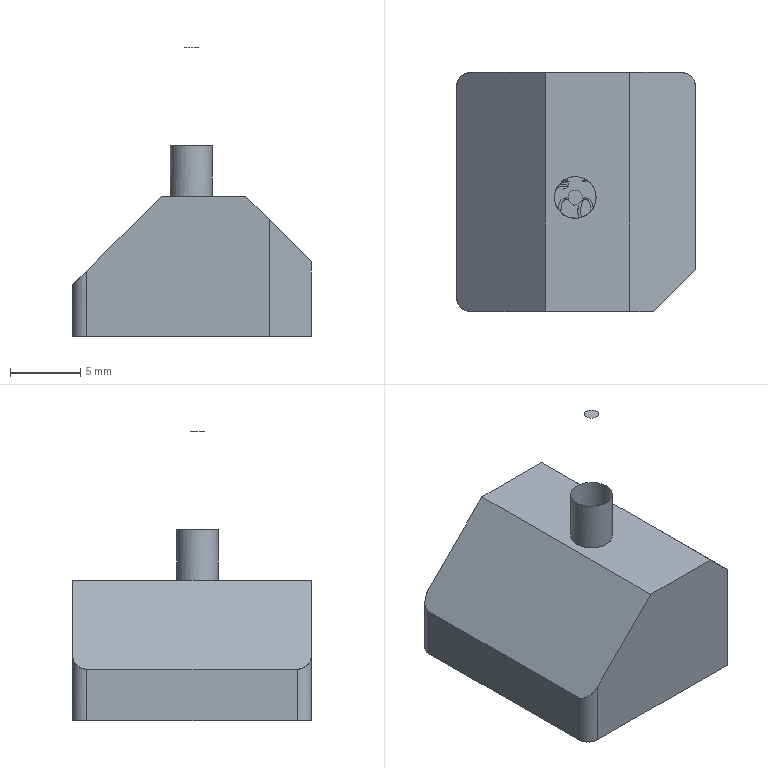NC program | PowerMill | posted with a generic post | part box 17 x 17 x 20.603 mm
Lines 3444 to 3961 of 42778:
N3541 M6
N3542 S8500 M03
N3543 G00 G90 X0.002 Y0.0
N3544 G43 Z11.803 H3
N3545
N3546 G05 P10000 R8
N3547 X6.5189 Y8.6331
N3548 Z0.8529
N3549 G01 Z-0.3471 F360.0
N3550 X3.4666 Y4.3309 F600.0
N3551 X-5.7661 Y-1.8674
N3552 X-5.6728 Y-2.1912
N3553 X-5.4516 Y-2.7818
N3554 X-5.3113 Y-3.0682
N3555 X-5.1953 Y-3.2909
N3556 X-4.9958 Y-3.6229
N3557 X-4.6728 Y-4.0697
N3558 X-4.5415 Y-4.2305
N3559 X-4.2593 Y-4.5375
N3560 G03 X-3.6303 Y-5.092 I4.7377 J4.7404
N3561 G01 X-3.5719 Y-5.1319
N3562 X5.661 Y1.0665
N3563 G00 Z11.803
N3564 G05 P0
N3565 (---------------)
N3566 ( END TOOLPATH : 粗公基准台01-平坦面平行-D10 )
N3567 (---------------)
N3568 ( START TOOLPATH : 粗公基准台01-基准面偏置-D10 )
N3569 (---------------)
N3570 G00 X0.002 Y0.0 Z9.8029
N3571 G05 P10000 R8
N3572 X-2.4609 Y19.1679
N3573 Z-9.6
N3574 G01 Z-10.8 F360.0
N3575 X-2.2639 Y13.8966 F600.0
N3576 X-5.1039 Y4.1284
N3577 G02 X-4.3127 Y4.8796 I6.1923 J-5.7295
N3578 G01 X-4.0577 Y5.0698
N3579 X-3.5215 Y5.4298
N3580 X-3.1259 Y5.6451
N3581 X-2.7927 Y5.8019
N3582 G02 X-2.3057 Y5.99 I1.3954 J-2.888
N3583 G01 X-1.9392 Y6.1117
N3584 G02 X-1.148 Y6.2935 I1.8874 J-6.3997
N3585 G01 X-0.3568 Y6.3775
N3586 X0.4344 Y6.3644
N3587 X0.83 Y6.3263
N3588 X1.2256 Y6.2581
N3589 G02 X2.0168 Y6.06 I-1.3394 J-7.0312
N3590 G01 X2.415 Y5.9128
N3591 X2.808 Y5.7518
N3592 X3.2036 Y5.548
N3593 X3.5992 Y5.3157
N3594 X3.8789 Y5.1285
N3595 X4.3904 Y4.724
N3596 X4.5997 Y4.5366
N3597 X4.7999 Y4.3395
N3598 X5.1816 Y3.9134
N3599 X5.462 Y3.5505
N3600 X5.72 Y3.156
N3601 X5.9727 Y2.7176
N3602 X6.3019 Y1.9725
N3603 X6.4361 Y1.578
N3604 X6.5399 Y1.1835
N3605 X6.6264 Y0.789
N3606 X6.6836 Y0.3945
N3607 X6.7315 Y-0.3945
N3608 X6.6843 Y-1.1835
N3609 X6.6285 Y-1.578
N3610 X6.5422 Y-1.9725
N3611 X6.4395 Y-2.367
N3612 X6.3065 Y-2.7615
N3613 X5.9557 Y-3.5505
N3614 X5.7269 Y-3.945
N3615 X5.4697 Y-4.3395
N3616 X5.1815 Y-4.7132
N3617 X4.8107 Y-5.1285
N3618 X4.6054 Y-5.3313
N3619 X4.3904 Y-5.5238
N3620 X3.8943 Y-5.9175
N3621 X3.5992 Y-6.1163
N3622 G02 X2.808 Y-6.5516 I-4.9668 J8.09
N3623 G01 X2.4155 Y-6.7137
N3624 X2.0168 Y-6.8598
N3625 X1.6212 Y-6.9736
N3626 X1.2256 Y-7.0586
N3627 X0.83 Y-7.1267
N3628 X0.4344 Y-7.1642
N3629 X-0.3568 Y-7.1773
N3630 X-1.148 Y-7.0933
N3631 G02 X-2.1733 Y-6.8331 I0.9602 J5.9347
N3632 G01 X-2.5519 Y-6.7065
N3633 X-3.126 Y-6.4452
N3634 X-3.5215 Y-6.2296
N3635 X-3.9929 Y-5.9175
N3636 X-4.3128 Y-5.6794
N3637 X-4.6133 Y-5.4182
N3638 X-4.9139 Y-5.1285
N3639 G02 X-5.5147 Y-4.4156 I4.536 J4.4326
N3640 G01 X-5.6438 Y-4.2299
N3641 X-5.8951 Y-3.8456
N3642 X-6.0842 Y-3.4937
N3643 X-6.2596 Y-3.1348
N3644 X-6.4097 Y-2.7615
N3645 X-6.5425 Y-2.367
N3646 X-6.6515 Y-1.9725
N3647 X-6.6863 Y-1.8138
N3648 X-6.7899 Y-1.1835
N3649 X-6.8246 Y-0.789
N3650 X-6.8313 Y-0.3945
N3651 X-6.8246 Y0.0
N3652 X-6.7883 Y0.3945
N3653 X-6.6767 Y1.064
N3654 X-6.5387 Y1.578
N3655 G02 X-6.2464 Y2.367 I7.6007 J-2.3668
N3656 G01 X-6.0757 Y2.709
N3657 X-5.8951 Y3.0458
N3658 X-5.7359 Y3.3024
N3659 X-5.5637 Y3.5505
N3660 X-5.3461 Y3.8394
N3661 X-5.1039 Y4.1284
N3662 G00 Z9.8029
N3663 G05 P0
N3664 (---------------)
N3665 ( END TOOLPATH : 粗公基准台01-基准面偏置-D10 )
N3666 (---------------)
N3667 ( START TOOLPATH : 粗公基准台01-基准台侧光-D10 )
N3668 (---------------)
N3669 G00 X0.002 Y0.0 Z9.8029
N3670 G05 P10000 R8
N3671 X13.4802 Y-14.7763
N3672 Z-19.5
N3673 G01 Z-20.7 F360.0
N3674 G03 X9.9447 Y-11.2408 I-1.7677 J1.7678 F600.0
N3675 G01 X9.0603 Y-12.1252
N3676 X9.0598 Y-12.1257
N3677 X9.0593 Y-12.1262
N3678 X8.9973 Y-12.186
N3679 X8.9953 Y-12.1879
N3680 X8.9933 Y-12.1896
N3681 X8.5463 Y-12.5663
N3682 X8.5428 Y-12.5691
N3683 X8.5391 Y-12.5717
N3684 X8.0921 Y-12.8697
N3685 X8.0892 Y-12.8716
N3686 X8.0862 Y-12.8734
N3687 X7.7951 Y-13.0328
N3688 X7.7933 Y-13.0337
N3689 X7.7915 Y-13.0346
N3690 X7.6356 Y-13.11
N3691 X7.6332 Y-13.1111
N3692 X7.6308 Y-13.1122
N3693 X7.1838 Y-13.2933
N3694 X7.1803 Y-13.2947
N3695 X7.1766 Y-13.2958
N3696 X6.7297 Y-13.4292
N3697 X6.7268 Y-13.43
N3698 X6.724 Y-13.4307
N3699 X6.4655 Y-13.4877
N3700 X6.4637 Y-13.4881
N3701 X6.4619 Y-13.4884
N3702 X6.2734 Y-13.521
N3703 X6.2709 Y-13.5214
N3704 X6.2684 Y-13.5217
N3705 X5.8214 Y-13.5699
N3706 X5.818 Y-13.5702
N3707 X5.8146 Y-13.5703
N3708 X5.3676 Y-13.58
N3709 X5.3667
N3710 X5.3658
N3711 X-7.5968 Y-13.5791
N3712 X-7.599 Y-13.579
N3713 X-7.6012 Y-13.5789
N3714 X-8.0482 Y-13.5541
N3715 X-8.0511 Y-13.5539
N3716 X-8.0539 Y-13.5536
N3717 X-8.5009 Y-13.4962
N3718 X-8.5039 Y-13.4958
N3719 X-8.5069 Y-13.4952
N3720 X-8.9539 Y-13.403
N3721 X-8.957 Y-13.4023
N3722 X-8.9601 Y-13.4014
N3723 X-9.4071 Y-13.271
N3724 X-9.4099 Y-13.2702
N3725 X-9.4126 Y-13.2692
N3726 X-9.8596 Y-13.1027
N3727 X-9.8628 Y-13.1014
N3728 X-9.866 Y-13.1
N3729 X-10.3129 Y-12.8881
N3730 X-10.3158 Y-12.8867
N3731 X-10.3186 Y-12.8851
N3732 X-10.7656 Y-12.6274
N3733 X-10.7687 Y-12.6256
N3734 X-10.7717 Y-12.6235
N3735 X-11.2187 Y-12.3088
N3736 X-11.2209 Y-12.3072
N3737 X-11.2231 Y-12.3055
N3738 X-11.4383 Y-12.1307
N3739 X-11.4399 Y-12.1294
N3740 X-11.4414 Y-12.1281
N3741 X-11.6731 Y-11.9195
N3742 X-11.6747 Y-11.9181
N3743 X-11.6762 Y-11.9166
N3744 X-11.9146 Y-11.6782
N3745 X-11.9161 Y-11.6767
N3746 X-11.9175 Y-11.6751
N3747 X-12.1261 Y-11.4435
N3748 X-12.1274 Y-11.4419
N3749 X-12.1287 Y-11.4404
N3750 X-12.3036 Y-11.2251
N3751 X-12.3052 Y-11.2231
N3752 X-12.3066 Y-11.2211
N3753 X-12.5787 Y-10.8401
N3754 X-12.5807 Y-10.8371
N3755 X-12.5826 Y-10.834
N3756 X-12.8831 Y-10.3211
N3757 X-12.8848 Y-10.3181
N3758 X-12.8863 Y-10.3149
N3759 X-13.0983 Y-9.868
N3760 X-13.0997 Y-9.8648
N3761 X-13.1009 Y-9.8616
N3762 X-13.2675 Y-9.4146
N3763 X-13.2685 Y-9.4119
N3764 X-13.2693 Y-9.4091
N3765 X-13.3997 Y-8.9621
N3766 X-13.4005 Y-8.9592
N3767 X-13.4012 Y-8.9562
N3768 X-13.4858 Y-8.555
N3769 X-13.4864 Y-8.552
N3770 X-13.4869 Y-8.549
N3771 X-13.552 Y-8.0562
N3772 X-13.5523 Y-8.0532
N3773 X-13.5525 Y-8.0502
N3774 X-13.5774 Y-7.6032
N3775 X-13.5775 Y-7.601
N3776 Y-7.5988
N3777 Y7.5988
N3778 Y7.601
N3779 X-13.5774 Y7.6032
N3780 X-13.5525 Y8.0502
N3781 X-13.5523 Y8.0531
N3782 X-13.552 Y8.0559
N3783 X-13.4946 Y8.5029
N3784 X-13.4941 Y8.5059
N3785 X-13.4936 Y8.5089
N3786 X-13.4013 Y8.9559
N3787 X-13.4005 Y8.959
N3788 X-13.3997 Y8.9621
N3789 X-13.2693 Y9.4091
N3790 X-13.2685 Y9.4119
N3791 X-13.2675 Y9.4146
N3792 X-13.1009 Y9.8616
N3793 X-13.0997 Y9.8648
N3794 X-13.0983 Y9.868
N3795 X-12.8863 Y10.3149
N3796 X-12.8849 Y10.3178
N3797 X-12.8834 Y10.3206
N3798 X-12.6256 Y10.7676
N3799 X-12.6237 Y10.7707
N3800 X-12.6217 Y10.7737
N3801 X-12.3069 Y11.2207
N3802 X-12.3053 Y11.2229
N3803 X-12.3036 Y11.2251
N3804 X-12.1287 Y11.4404
N3805 X-12.1274 Y11.4419
N3806 X-12.1261 Y11.4435
N3807 X-11.9175 Y11.6751
N3808 X-11.9161 Y11.6767
N3809 X-11.9146 Y11.6782
N3810 X-11.6762 Y11.9166
N3811 X-11.6747 Y11.9181
N3812 X-11.6731 Y11.9195
N3813 X-11.4414 Y12.1281
N3814 X-11.4399 Y12.1294
N3815 X-11.4383 Y12.1307
N3816 X-11.2231 Y12.3055
N3817 X-11.2211 Y12.3071
N3818 X-11.2191 Y12.3085
N3819 X-10.8379 Y12.5807
N3820 X-10.8349 Y12.5827
N3821 X-10.8318 Y12.5846
N3822 X-10.3191 Y12.8849
N3823 X-10.3161 Y12.8865
N3824 X-10.3129 Y12.8881
N3825 X-9.866 Y13.1
N3826 X-9.8628 Y13.1014
N3827 X-9.8596 Y13.1027
N3828 X-9.4126 Y13.2692
N3829 X-9.4099 Y13.2702
N3830 X-9.4071 Y13.271
N3831 X-8.9601 Y13.4014
N3832 X-8.9572 Y13.4022
N3833 X-8.9542 Y13.4029
N3834 X-8.5509 Y13.4879
N3835 X-8.5479 Y13.4884
N3836 X-8.5449 Y13.4889
N3837 X-8.0542 Y13.5535
N3838 X-8.0512 Y13.5539
N3839 X-8.0482 Y13.5541
N3840 X-7.6012 Y13.579
N3841 X-7.599 Y13.5791
N3842 X-7.5968
N3843 X0.002
N3844 X7.6008 Y13.579
N3845 X7.603
N3846 X7.6052 Y13.5789
N3847 X8.0522 Y13.5541
N3848 X8.0551 Y13.5538
N3849 X8.0579 Y13.5535
N3850 X8.5049 Y13.4961
N3851 X8.5079 Y13.4956
N3852 X8.5109 Y13.4951
N3853 X8.9579 Y13.4027
N3854 X8.961 Y13.402
N3855 X8.9641 Y13.4012
N3856 X9.4111 Y13.2707
N3857 X9.4139 Y13.2699
N3858 X9.4166 Y13.2689
N3859 X9.8636 Y13.1024
N3860 X9.8668 Y13.1011
N3861 X9.87 Y13.0997
N3862 X10.317 Y12.8876
N3863 X10.3198 Y12.8862
N3864 X10.3226 Y12.8847
N3865 X10.7696 Y12.6269
N3866 X10.7727 Y12.625
N3867 X10.7757 Y12.623
N3868 X11.2227 Y12.3082
N3869 X11.2249 Y12.3066
N3870 X11.2271 Y12.3049
N3871 X11.4415 Y12.1307
N3872 X11.443 Y12.1294
N3873 X11.4446 Y12.1281
N3874 X11.6771 Y11.9187
N3875 X11.6787 Y11.9173
N3876 X11.6802 Y11.9158
N3877 X11.9178 Y11.6782
N3878 X11.9193 Y11.6767
N3879 X11.9207 Y11.6751
N3880 X12.1301 Y11.4424
N3881 X12.1314 Y11.4409
N3882 X12.1327 Y11.4394
N3883 X12.3068 Y11.2251
N3884 X12.3083 Y11.2231
N3885 X12.3098 Y11.2211
N3886 X12.5827 Y10.8388
N3887 X12.5847 Y10.8358
N3888 X12.5866 Y10.8327
N3889 X12.8862 Y10.3211
N3890 X12.8879 Y10.3181
N3891 X12.8895 Y10.3149
N3892 X13.1014 Y9.868
N3893 X13.1028 Y9.8648
N3894 X13.1041 Y9.8616
N3895 X13.2706 Y9.4146
N3896 X13.2716 Y9.4119
N3897 X13.2725 Y9.4091
N3898 X13.4029 Y8.9621
N3899 X13.4037 Y8.9592
N3900 X13.4044 Y8.9562
N3901 X13.4899 Y8.55
N3902 X13.4904 Y8.547
N3903 X13.4909 Y8.5439
N3904 X13.5551 Y8.0562
N3905 X13.5554 Y8.0532
N3906 X13.5556 Y8.0502
N3907 X13.5805 Y7.6032
N3908 X13.5806 Y7.601
N3909 Y7.5988
N3910 X13.5816 Y-5.3638
N3911 Y-5.3647
N3912 Y-5.3656
N3913 X13.5719 Y-5.8126
N3914 X13.5717 Y-5.816
N3915 X13.5715 Y-5.8194
N3916 X13.5234 Y-6.2664
N3917 X13.5231 Y-6.2689
N3918 X13.5227 Y-6.2714
N3919 X13.4904 Y-6.4581
N3920 X13.4901 Y-6.4599
N3921 X13.4897 Y-6.4616
N3922 X13.4324 Y-6.722
N3923 X13.4317 Y-6.7248
N3924 X13.431 Y-6.7277
N3925 X13.2975 Y-7.1747
N3926 X13.2964 Y-7.1783
N3927 X13.295 Y-7.1818
N3928 X13.1139 Y-7.6288
N3929 X13.1129 Y-7.6312
N3930 X13.1118 Y-7.6336
N3931 X13.0366 Y-7.7891
N3932 X13.0357 Y-7.7909
N3933 X13.0348 Y-7.7926
N3934 X12.8752 Y-8.0842
N3935 X12.8735 Y-8.0871
N3936 X12.8716 Y-8.09
N3937 X12.5842 Y-8.5228
N3938 X12.5817 Y-8.5265
N3939 X12.5789 Y-8.53
N3940 X12.1917 Y-8.9912
N3941 X12.1899 Y-8.9932
N3942 X12.188 Y-8.9953
N3943 X12.1282 Y-9.0573
N3944 X12.1277 Y-9.0578
N3945 X12.1272 Y-9.0583
N3946 X9.9447 Y-11.2408
N3947 G03 X13.4802 Y-14.7763 I1.7678 J-1.7677
N3948 G01 X13.4288 Y-14.7146
N3949 G03 X9.8932 Y-11.1791 I-1.7678 J1.7677
N3950 G01 X9.0037 Y-12.0686
N3951 X8.9417 Y-12.1285
N3952 X8.4947 Y-12.5052
N3953 X8.0477 Y-12.8032
N3954 X7.7566 Y-12.9626
N3955 X7.6008 Y-13.038
N3956 X7.1538 Y-13.2192
N3957 X6.7068 Y-13.3526
N3958 X6.4482 Y-13.4096
N3959 X6.2598 Y-13.4422
N3960 X5.8128 Y-13.4903
N3961 X5.3658 Y-13.5
N3962 X-7.5968 Y-13.4991
N3963 X-8.0437 Y-13.4742
N3964 X-8.4907 Y-13.4169
N3965 X-8.9377 Y-13.3246
N3966 X-9.3847 Y-13.1942
N3967 X-9.8317 Y-13.0277
N3968 X-10.2787 Y-12.8158
N3969 X-10.7257 Y-12.5581
N3970 X-11.1726 Y-12.2434
N3971 X-11.3879 Y-12.0686
N3972 X-11.6196 Y-11.8601
N3973 X-11.8581 Y-11.6216
N3974 X-12.0666 Y-11.3899
N3975 X-12.2415 Y-11.1746
N3976 X-12.5136 Y-10.7936
N3977 X-12.8141 Y-10.2807
N3978 X-13.026 Y-9.8337
N3979 X-13.1925 Y-9.3867
N3980 X-13.3229 Y-8.9397
N3981 X-13.4076 Y-8.5385
N3982 X-13.4726 Y-8.0457
N3983 X-13.4975 Y-7.5988
N3984 Y7.5988
N3985 X-13.4726 Y8.0457
N3986 X-13.4152 Y8.4927
N3987 X-13.3229 Y8.9397
N3988 X-13.1925 Y9.3867
N3989 X-13.026 Y9.8337
N3990 X-12.8141 Y10.2807
N3991 X-12.5563 Y10.7277
N3992 X-12.2415 Y11.1746
N3993 X-12.0666 Y11.3899
N3994 X-11.8581 Y11.6216
N3995 X-11.6196 Y11.8601
N3996 X-11.3879 Y12.0686
N3997 X-11.1726 Y12.2434
N3998 X-10.7914 Y12.5156
N3999 X-10.2787 Y12.8158
N4000 X-9.8317 Y13.0277
N4001 X-9.3847 Y13.1942
N4002 X-8.9377 Y13.3246
N4003 X-8.5344 Y13.4096
N4004 X-8.0437 Y13.4742
N4005 X-7.5968 Y13.4991
N4006 X0.002
N4007 X7.6008 Y13.499
N4008 X8.0477 Y13.4742
N4009 X8.4947 Y13.4167
N4010 X8.9417 Y13.3244
N4011 X9.3887 Y13.1939
N4012 X9.8357 Y13.0274
N4013 X10.2827 Y12.8154
N4014 X10.7297 Y12.5576
N4015 X11.1766 Y12.2428
N4016 X11.391 Y12.0686
N4017 X11.6236 Y11.8593
N4018 X11.8612 Y11.6216
N4019 X12.0706 Y11.3889
N4020 X12.2447 Y11.1746
N4021 X12.5176 Y10.7923
N4022 X12.8172 Y10.2807
N4023 X13.0291 Y9.8337
N4024 X13.1957 Y9.3867
N4025 X13.3261 Y8.9397
N4026 X13.4116 Y8.5335
N4027 X13.4758 Y8.0457
N4028 X13.5006 Y7.5988
N4029 X13.5016 Y-5.3638
N4030 X13.4919 Y-5.8108
N4031 X13.4439 Y-6.2578
N4032 X13.4116 Y-6.4444
N4033 X13.3543 Y-6.7048
N4034 X13.2209 Y-7.1518
N4035 X13.0398 Y-7.5988
N4036 X12.9646 Y-7.7542
N4037 X12.805 Y-8.0457
N4038 X12.5176 Y-8.4786
N4039 X12.1304 Y-8.9397
N4040 X12.0706 Y-9.0017
N4041 X9.8932 Y-11.1791
N4042 G03 X13.4288 Y-14.7146 I1.7678 J-1.7678
N4043 G00 Z9.8029
N4044 G05 P0
N4045 (---------------)
N4046 ( END TOOLPATH : 粗公基准台01-基准台侧光-D10 )
N4047 (---------------)
N4048
N4049 M05
N4050 G53 Z0.0
N4051 (---------------)
N4052 ( START TOOLPATH : 粗公精光01-等高-D4 )
N4053 (---------------)
N4054 ( TOOL NO.    :14 )
N4055 ( TOOL TYPE   : ENDMILL)
N4056 ( TOOL ID     : D4_2_1)
N4057 ( TOOL DIA    : 4.0 LENGTH 65.68)
N4058 T14